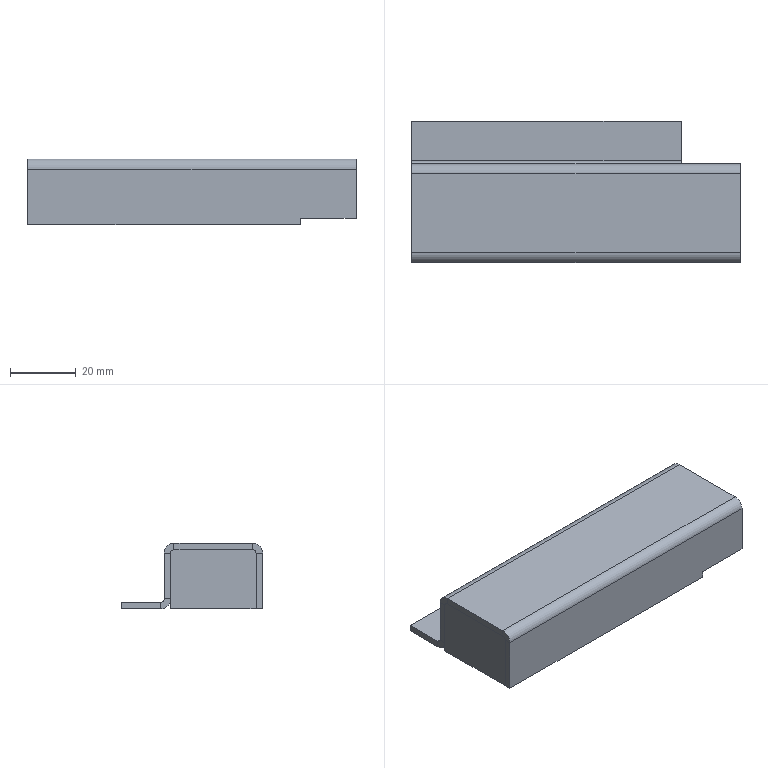Part | SolidWorks | features BaseBody 2 | 2 solids | 44 faces | box 100 x 43 x 20 mm | volume 15639 mm3 | plane 36 | cylinder 8 | commonest cylinder face diameters 2 x5 6 x3
STEP:
#1=CARTESIAN_POINT('',(33.,-13.,-20.));
#2=VERTEX_POINT('',#1);
#3=CARTESIAN_POINT('',(33.,-13.,-18.));
#4=VERTEX_POINT('',#3);
#5=CARTESIAN_POINT('',(33.,-13.,0.));
#6=DIRECTION('',(0.,0.,1.));
#7=VECTOR('',#6,1000.);
#8=LINE('',#5,#7);
#9=EDGE_CURVE('',#2,#4,#8,.T.);
#10=ORIENTED_EDGE('',*,*,#9,.T.);
#11=CARTESIAN_POINT('',(33.,-15.,-18.));
#12=VERTEX_POINT('',#11);
#13=CARTESIAN_POINT('',(33.,-15.,-18.));
#14=DIRECTION('',(0.,1.,0.));
#15=VECTOR('',#14,1000.);
#16=LINE('',#13,#15);
#17=EDGE_CURVE('',#12,#4,#16,.T.);
#18=ORIENTED_EDGE('',*,*,#17,.F.);
#19=CARTESIAN_POINT('',(33.,-15.,-20.));
#20=VERTEX_POINT('',#19);
#21=CARTESIAN_POINT('',(33.,-15.,-20.));
#22=DIRECTION('',(0.,0.,1.));
#23=VECTOR('',#22,1000.);
#24=LINE('',#21,#23);
#25=EDGE_CURVE('',#20,#12,#24,.T.);
#26=ORIENTED_EDGE('',*,*,#25,.F.);
#27=CARTESIAN_POINT('',(33.,-15.,-20.));
#28=DIRECTION('',(0.,1.,0.));
#29=VECTOR('',#28,1000.);
#30=LINE('',#27,#29);
#31=EDGE_CURVE('',#20,#2,#30,.T.);
#32=ORIENTED_EDGE('',*,*,#31,.T.);
#33=EDGE_LOOP('',(#10,#18,#26,#32));
#34=FACE_OUTER_BOUND('',#33,.T.);
#35=CARTESIAN_POINT('',(33.,-15.,-20.));
#36=DIRECTION('',(-1.,0.,0.));
#37=DIRECTION('',(0.,0.,1.));
#38=AXIS2_PLACEMENT_3D('',#35,#36,#37);
#39=PLANE('',#38);
#40=ADVANCED_FACE('',(#34),#39,.F.);
#41=CARTESIAN_POINT('',(50.,-13.,-18.));
#42=VERTEX_POINT('',#41);
#43=CARTESIAN_POINT('',(0.,-13.,-18.));
#44=DIRECTION('',(1.,0.,0.));
#45=VECTOR('',#44,1000.);
#46=LINE('',#43,#45);
#47=EDGE_CURVE('',#4,#42,#46,.T.);
#48=ORIENTED_EDGE('',*,*,#47,.T.);
#49=CARTESIAN_POINT('',(50.,-15.,-18.));
#50=VERTEX_POINT('',#49);
#51=CARTESIAN_POINT('',(50.,-15.,-18.));
#52=DIRECTION('',(0.,1.,0.));
#53=VECTOR('',#52,1000.);
#54=LINE('',#51,#53);
#55=EDGE_CURVE('',#50,#42,#54,.T.);
#56=ORIENTED_EDGE('',*,*,#55,.F.);
#57=CARTESIAN_POINT('',(50.,-15.,-18.));
#58=DIRECTION('',(1.,0.,0.));
#59=VECTOR('',#58,1000.);
#60=LINE('',#57,#59);
#61=EDGE_CURVE('',#12,#50,#60,.T.);
#62=ORIENTED_EDGE('',*,*,#61,.F.);
#63=ORIENTED_EDGE('',*,*,#17,.T.);
#64=EDGE_LOOP('',(#48,#56,#62,#63));
#65=FACE_OUTER_BOUND('',#64,.T.);
#66=CARTESIAN_POINT('',(50.,-15.,-18.));
#67=DIRECTION('',(0.,0.,1.));
#68=DIRECTION('',(0.,-1.,0.));
#69=AXIS2_PLACEMENT_3D('',#66,#67,#68);
#70=PLANE('',#69);
#71=ADVANCED_FACE('',(#65),#70,.F.);
#72=CARTESIAN_POINT('',(33.,13.,-18.));
#73=VERTEX_POINT('',#72);
#74=CARTESIAN_POINT('',(33.,15.,-18.));
#75=VERTEX_POINT('',#74);
#76=CARTESIAN_POINT('',(33.,15.,-18.));
#77=DIRECTION('',(0.,1.,0.));
#78=VECTOR('',#77,1000.);
#79=LINE('',#76,#78);
#80=EDGE_CURVE('',#73,#75,#79,.T.);
#81=ORIENTED_EDGE('',*,*,#80,.T.);
#82=CARTESIAN_POINT('',(50.,15.,-18.));
#83=VERTEX_POINT('',#82);
#84=CARTESIAN_POINT('',(50.,15.,-18.));
#85=DIRECTION('',(1.,0.,0.));
#86=VECTOR('',#85,1000.);
#87=LINE('',#84,#86);
#88=EDGE_CURVE('',#75,#83,#87,.T.);
#89=ORIENTED_EDGE('',*,*,#88,.T.);
#90=CARTESIAN_POINT('',(50.,13.,-18.));
#91=VERTEX_POINT('',#90);
#92=CARTESIAN_POINT('',(50.,-15.,-18.));
#93=DIRECTION('',(0.,1.,0.));
#94=VECTOR('',#93,1000.);
#95=LINE('',#92,#94);
#96=EDGE_CURVE('',#91,#83,#95,.T.);
#97=ORIENTED_EDGE('',*,*,#96,.F.);
#98=CARTESIAN_POINT('',(0.,13.,-18.));
#99=DIRECTION('',(1.,0.,0.));
#100=VECTOR('',#99,1000.);
#101=LINE('',#98,#100);
#102=EDGE_CURVE('',#73,#91,#101,.T.);
#103=ORIENTED_EDGE('',*,*,#102,.F.);
#104=EDGE_LOOP('',(#81,#89,#97,#103));
#105=FACE_OUTER_BOUND('',#104,.T.);
#106=CARTESIAN_POINT('',(50.,-15.,-18.));
#107=DIRECTION('',(0.,0.,1.));
#108=DIRECTION('',(0.,-1.,0.));
#109=AXIS2_PLACEMENT_3D('',#106,#107,#108);
#110=PLANE('',#109);
#111=ADVANCED_FACE('',(#105),#110,.F.);
#112=CARTESIAN_POINT('',(32.,28.,-18.));
#113=VERTEX_POINT('',#112);
#114=CARTESIAN_POINT('',(-50.,28.,-18.));
#115=VERTEX_POINT('',#114);
#116=CARTESIAN_POINT('',(0.,28.,-18.));
#117=DIRECTION('',(-1.,0.,0.));
#118=VECTOR('',#117,1000.);
#119=LINE('',#116,#118);
#120=EDGE_CURVE('',#113,#115,#119,.T.);
#121=ORIENTED_EDGE('',*,*,#120,.F.);
#122=CARTESIAN_POINT('',(32.,28.,-20.));
#123=VERTEX_POINT('',#122);
#124=CARTESIAN_POINT('',(32.,28.,-20.));
#125=DIRECTION('',(0.,0.,1.));
#126=VECTOR('',#125,1000.);
#127=LINE('',#124,#126);
#128=EDGE_CURVE('',#123,#113,#127,.T.);
#129=ORIENTED_EDGE('',*,*,#128,.F.);
#130=CARTESIAN_POINT('',(-50.,28.,-20.));
#131=VERTEX_POINT('',#130);
#132=CARTESIAN_POINT('',(-50.,28.,-20.));
#133=DIRECTION('',(-1.,0.,0.));
#134=VECTOR('',#133,1000.);
#135=LINE('',#132,#134);
#136=EDGE_CURVE('',#123,#131,#135,.T.);
#137=ORIENTED_EDGE('',*,*,#136,.T.);
#138=CARTESIAN_POINT('',(-50.,28.,-20.));
#139=DIRECTION('',(0.,0.,1.));
#140=VECTOR('',#139,1000.);
#141=LINE('',#138,#140);
#142=EDGE_CURVE('',#131,#115,#141,.T.);
#143=ORIENTED_EDGE('',*,*,#142,.T.);
#144=EDGE_LOOP('',(#121,#129,#137,#143));
#145=FACE_OUTER_BOUND('',#144,.T.);
#146=CARTESIAN_POINT('',(-50.,28.,-20.));
#147=DIRECTION('',(0.,1.,0.));
#148=DIRECTION('',(1.,0.,0.));
#149=AXIS2_PLACEMENT_3D('',#146,#147,#148);
#150=PLANE('',#149);
#151=ADVANCED_FACE('',(#145),#150,.T.);
#152=CARTESIAN_POINT('',(32.,16.,-18.));
#153=VERTEX_POINT('',#152);
#154=CARTESIAN_POINT('',(-50.,16.,-18.));
#155=VERTEX_POINT('',#154);
#156=CARTESIAN_POINT('',(32.,16.,-18.));
#157=DIRECTION('',(-1.,0.,0.));
#158=VECTOR('',#157,1000.);
#159=LINE('',#156,#158);
#160=EDGE_CURVE('',#153,#155,#159,.T.);
#161=ORIENTED_EDGE('',*,*,#160,.F.);
#162=CARTESIAN_POINT('',(32.,0.,-18.));
#163=DIRECTION('',(0.,1.,0.));
#164=VECTOR('',#163,1000.);
#165=LINE('',#162,#164);
#166=EDGE_CURVE('',#153,#113,#165,.T.);
#167=ORIENTED_EDGE('',*,*,#166,.T.);
#168=ORIENTED_EDGE('',*,*,#120,.T.);
#169=CARTESIAN_POINT('',(-50.,0.,-18.));
#170=DIRECTION('',(0.,-1.,0.));
#171=VECTOR('',#170,1000.);
#172=LINE('',#169,#171);
#173=EDGE_CURVE('',#115,#155,#172,.T.);
#174=ORIENTED_EDGE('',*,*,#173,.T.);
#175=EDGE_LOOP('',(#161,#167,#168,#174));
#176=FACE_OUTER_BOUND('',#175,.T.);
#177=CARTESIAN_POINT('',(0.,0.,-18.));
#178=DIRECTION('',(0.,0.,-1.));
#179=DIRECTION('',(0.,-1.,0.));
#180=AXIS2_PLACEMENT_3D('',#177,#178,#179);
#181=PLANE('',#180);
#182=ADVANCED_FACE('',(#176),#181,.F.);
#183=CARTESIAN_POINT('',(32.,16.,-20.));
#184=VERTEX_POINT('',#183);
#185=CARTESIAN_POINT('',(32.,15.,-20.));
#186=DIRECTION('',(0.,1.,0.));
#187=VECTOR('',#186,1000.);
#188=LINE('',#185,#187);
#189=EDGE_CURVE('',#184,#123,#188,.T.);
#190=ORIENTED_EDGE('',*,*,#189,.F.);
#191=CARTESIAN_POINT('',(-50.,16.,-20.));
#192=VERTEX_POINT('',#191);
#193=CARTESIAN_POINT('',(0.,16.,-20.));
#194=DIRECTION('',(-1.,0.,0.));
#195=VECTOR('',#194,1000.);
#196=LINE('',#193,#195);
#197=EDGE_CURVE('',#184,#192,#196,.T.);
#198=ORIENTED_EDGE('',*,*,#197,.T.);
#199=CARTESIAN_POINT('',(-50.,15.,-20.));
#200=DIRECTION('',(0.,-1.,0.));
#201=VECTOR('',#200,1000.);
#202=LINE('',#199,#201);
#203=EDGE_CURVE('',#131,#192,#202,.T.);
#204=ORIENTED_EDGE('',*,*,#203,.F.);
#205=ORIENTED_EDGE('',*,*,#136,.F.);
#206=EDGE_LOOP('',(#190,#198,#204,#205));
#207=FACE_OUTER_BOUND('',#206,.T.);
#208=CARTESIAN_POINT('',(0.,0.,-20.));
#209=DIRECTION('',(0.,0.,-1.));
#210=DIRECTION('',(0.,-1.,0.));
#211=AXIS2_PLACEMENT_3D('',#208,#209,#210);
#212=PLANE('',#211);
#213=ADVANCED_FACE('',(#207),#212,.T.);
#214=ORIENTED_EDGE('',*,*,#166,.F.);
#215=CARTESIAN_POINT('',(32.,16.,-20.));
#216=DIRECTION('',(0.,0.,-1.));
#217=VECTOR('',#216,1000.);
#218=LINE('',#215,#217);
#219=EDGE_CURVE('',#153,#184,#218,.T.);
#220=ORIENTED_EDGE('',*,*,#219,.T.);
#221=ORIENTED_EDGE('',*,*,#189,.T.);
#222=ORIENTED_EDGE('',*,*,#128,.T.);
#223=EDGE_LOOP('',(#214,#220,#221,#222));
#224=FACE_OUTER_BOUND('',#223,.T.);
#225=CARTESIAN_POINT('',(32.,15.,-20.));
#226=DIRECTION('',(1.,0.,0.));
#227=DIRECTION('',(0.,1.,0.));
#228=AXIS2_PLACEMENT_3D('',#225,#226,#227);
#229=PLANE('',#228);
#230=ADVANCED_FACE('',(#224),#229,.T.);
#231=ORIENTED_EDGE('',*,*,#203,.T.);
#232=CARTESIAN_POINT('',(-50.,16.,-18.));
#233=DIRECTION('',(0.,0.,-1.));
#234=VECTOR('',#233,1000.);
#235=LINE('',#232,#234);
#236=EDGE_CURVE('',#155,#192,#235,.T.);
#237=ORIENTED_EDGE('',*,*,#236,.F.);
#238=ORIENTED_EDGE('',*,*,#173,.F.);
#239=ORIENTED_EDGE('',*,*,#142,.F.);
#240=EDGE_LOOP('',(#231,#237,#238,#239));
#241=FACE_OUTER_BOUND('',#240,.T.);
#242=CARTESIAN_POINT('',(-50.,15.,-20.));
#243=DIRECTION('',(-1.,0.,0.));
#244=DIRECTION('',(0.,0.,1.));
#245=AXIS2_PLACEMENT_3D('',#242,#243,#244);
#246=PLANE('',#245);
#247=ADVANCED_FACE('',(#241),#246,.T.);
#248=CARTESIAN_POINT('',(-50.,15.,-17.));
#249=VERTEX_POINT('',#248);
#250=CARTESIAN_POINT('',(32.,15.,-17.));
#251=VERTEX_POINT('',#250);
#252=CARTESIAN_POINT('',(-50.,15.,-17.));
#253=DIRECTION('',(1.,0.,0.));
#254=VECTOR('',#253,1000.);
#255=LINE('',#252,#254);
#256=EDGE_CURVE('',#249,#251,#255,.T.);
#257=ORIENTED_EDGE('',*,*,#256,.T.);
#258=CARTESIAN_POINT('',(32.,16.,-17.));
#259=DIRECTION('',(1.,0.,0.));
#260=DIRECTION('',(0.,0.,1.));
#261=AXIS2_PLACEMENT_3D('',#258,#259,#260);
#262=CIRCLE('',#261,1.);
#263=EDGE_CURVE('',#251,#153,#262,.T.);
#264=ORIENTED_EDGE('',*,*,#263,.T.);
#265=ORIENTED_EDGE('',*,*,#160,.T.);
#266=CARTESIAN_POINT('',(-50.,16.,-17.));
#267=DIRECTION('',(-1.,0.,0.));
#268=DIRECTION('',(0.,0.,1.));
#269=AXIS2_PLACEMENT_3D('',#266,#267,#268);
#270=CIRCLE('',#269,1.);
#271=EDGE_CURVE('',#155,#249,#270,.T.);
#272=ORIENTED_EDGE('',*,*,#271,.T.);
#273=EDGE_LOOP('',(#257,#264,#265,#272));
#274=FACE_OUTER_BOUND('',#273,.T.);
#275=CARTESIAN_POINT('',(-50.,16.,-17.));
#276=DIRECTION('',(-1.,0.,0.));
#277=DIRECTION('',(0.,0.,-1.));
#278=AXIS2_PLACEMENT_3D('',#275,#276,#277);
#279=CYLINDRICAL_SURFACE('',#278,1.);
#280=ADVANCED_FACE('',(#274),#279,.F.);
#281=CARTESIAN_POINT('',(-50.,13.,-17.));
#282=VERTEX_POINT('',#281);
#283=CARTESIAN_POINT('',(32.,13.,-17.));
#284=VERTEX_POINT('',#283);
#285=CARTESIAN_POINT('',(-50.,13.,-17.));
#286=DIRECTION('',(1.,0.,0.));
#287=VECTOR('',#286,1000.);
#288=LINE('',#285,#287);
#289=EDGE_CURVE('',#282,#284,#288,.T.);
#290=ORIENTED_EDGE('',*,*,#289,.F.);
#291=CARTESIAN_POINT('',(-50.,16.,-17.));
#292=DIRECTION('',(-1.,0.,0.));
#293=DIRECTION('',(0.,0.,1.));
#294=AXIS2_PLACEMENT_3D('',#291,#292,#293);
#295=CIRCLE('',#294,3.);
#296=EDGE_CURVE('',#192,#282,#295,.T.);
#297=ORIENTED_EDGE('',*,*,#296,.F.);
#298=ORIENTED_EDGE('',*,*,#197,.F.);
#299=CARTESIAN_POINT('',(32.,16.,-17.));
#300=DIRECTION('',(1.,0.,0.));
#301=DIRECTION('',(0.,0.,1.));
#302=AXIS2_PLACEMENT_3D('',#299,#300,#301);
#303=CIRCLE('',#302,3.);
#304=EDGE_CURVE('',#284,#184,#303,.T.);
#305=ORIENTED_EDGE('',*,*,#304,.F.);
#306=EDGE_LOOP('',(#290,#297,#298,#305));
#307=FACE_OUTER_BOUND('',#306,.T.);
#308=CARTESIAN_POINT('',(-50.,16.,-17.));
#309=DIRECTION('',(-1.,0.,0.));
#310=DIRECTION('',(0.,0.,-1.));
#311=AXIS2_PLACEMENT_3D('',#308,#309,#310);
#312=CYLINDRICAL_SURFACE('',#311,3.);
#313=ADVANCED_FACE('',(#307),#312,.T.);
#314=ORIENTED_EDGE('',*,*,#271,.F.);
#315=ORIENTED_EDGE('',*,*,#236,.T.);
#316=ORIENTED_EDGE('',*,*,#296,.T.);
#317=CARTESIAN_POINT('',(-50.,15.,-17.));
#318=DIRECTION('',(0.,-1.,0.));
#319=VECTOR('',#318,1000.);
#320=LINE('',#317,#319);
#321=EDGE_CURVE('',#249,#282,#320,.T.);
#322=ORIENTED_EDGE('',*,*,#321,.F.);
#323=EDGE_LOOP('',(#314,#315,#316,#322));
#324=FACE_OUTER_BOUND('',#323,.T.);
#325=CARTESIAN_POINT('',(-50.,16.,-17.));
#326=DIRECTION('',(1.,0.,0.));
#327=DIRECTION('',(0.,1.,0.));
#328=AXIS2_PLACEMENT_3D('',#325,#326,#327);
#329=PLANE('',#328);
#330=ADVANCED_FACE('',(#324),#329,.F.);
#331=ORIENTED_EDGE('',*,*,#219,.F.);
#332=ORIENTED_EDGE('',*,*,#263,.F.);
#333=CARTESIAN_POINT('',(32.,15.,-17.));
#334=DIRECTION('',(0.,-1.,0.));
#335=VECTOR('',#334,1000.);
#336=LINE('',#333,#335);
#337=EDGE_CURVE('',#251,#284,#336,.T.);
#338=ORIENTED_EDGE('',*,*,#337,.T.);
#339=ORIENTED_EDGE('',*,*,#304,.T.);
#340=EDGE_LOOP('',(#331,#332,#338,#339));
#341=FACE_OUTER_BOUND('',#340,.T.);
#342=CARTESIAN_POINT('',(32.,16.,-17.));
#343=DIRECTION('',(1.,0.,0.));
#344=DIRECTION('',(0.,1.,0.));
#345=AXIS2_PLACEMENT_3D('',#342,#343,#344);
#346=PLANE('',#345);
#347=ADVANCED_FACE('',(#341),#346,.T.);
#348=ORIENTED_EDGE('',*,*,#80,.F.);
#349=CARTESIAN_POINT('',(33.,13.,-16.));
#350=VERTEX_POINT('',#349);
#351=CARTESIAN_POINT('',(33.,13.,0.));
#352=DIRECTION('',(0.,0.,1.));
#353=VECTOR('',#352,1000.);
#354=LINE('',#351,#353);
#355=EDGE_CURVE('',#73,#350,#354,.T.);
#356=ORIENTED_EDGE('',*,*,#355,.T.);
#357=CARTESIAN_POINT('',(33.,15.,-16.));
#358=VERTEX_POINT('',#357);
#359=CARTESIAN_POINT('',(33.,15.,-16.));
#360=DIRECTION('',(0.,-1.,0.));
#361=VECTOR('',#360,1000.);
#362=LINE('',#359,#361);
#363=EDGE_CURVE('',#358,#350,#362,.T.);
#364=ORIENTED_EDGE('',*,*,#363,.F.);
#365=CARTESIAN_POINT('',(33.,15.,-16.));
#366=DIRECTION('',(0.,0.,-1.));
#367=VECTOR('',#366,1000.);
#368=LINE('',#365,#367);
#369=EDGE_CURVE('',#358,#75,#368,.T.);
#370=ORIENTED_EDGE('',*,*,#369,.T.);
#371=EDGE_LOOP('',(#348,#356,#364,#370));
#372=FACE_OUTER_BOUND('',#371,.T.);
#373=CARTESIAN_POINT('',(33.,15.,-16.));
#374=DIRECTION('',(-1.,0.,0.));
#375=DIRECTION('',(0.,0.,1.));
#376=AXIS2_PLACEMENT_3D('',#373,#374,#375);
#377=PLANE('',#376);
#378=ADVANCED_FACE('',(#372),#377,.T.);
#379=ORIENTED_EDGE('',*,*,#363,.T.);
#380=CARTESIAN_POINT('',(32.,13.,-16.));
#381=VERTEX_POINT('',#380);
#382=CARTESIAN_POINT('',(0.,13.,-16.));
#383=DIRECTION('',(-1.,0.,0.));
#384=VECTOR('',#383,1000.);
#385=LINE('',#382,#384);
#386=EDGE_CURVE('',#350,#381,#385,.T.);
#387=ORIENTED_EDGE('',*,*,#386,.T.);
#388=CARTESIAN_POINT('',(32.,15.,-16.));
#389=VERTEX_POINT('',#388);
#390=CARTESIAN_POINT('',(32.,15.,-16.));
#391=DIRECTION('',(0.,-1.,0.));
#392=VECTOR('',#391,1000.);
#393=LINE('',#390,#392);
#394=EDGE_CURVE('',#389,#381,#393,.T.);
#395=ORIENTED_EDGE('',*,*,#394,.F.);
#396=CARTESIAN_POINT('',(32.,15.,-16.));
#397=DIRECTION('',(1.,0.,0.));
#398=VECTOR('',#397,1000.);
#399=LINE('',#396,#398);
#400=EDGE_CURVE('',#389,#358,#399,.T.);
#401=ORIENTED_EDGE('',*,*,#400,.T.);
#402=EDGE_LOOP('',(#379,#387,#395,#401));
#403=FACE_OUTER_BOUND('',#402,.T.);
#404=CARTESIAN_POINT('',(32.,15.,-16.));
#405=DIRECTION('',(0.,0.,-1.));
#406=DIRECTION('',(-1.,0.,0.));
#407=AXIS2_PLACEMENT_3D('',#404,#405,#406);
#408=PLANE('',#407);
#409=ADVANCED_FACE('',(#403),#408,.T.);
#410=ORIENTED_EDGE('',*,*,#394,.T.);
#411=CARTESIAN_POINT('',(32.,13.,0.));
#412=DIRECTION('',(0.,0.,-1.));
#413=VECTOR('',#412,1000.);
#414=LINE('',#411,#413);
#415=EDGE_CURVE('',#381,#284,#414,.T.);
#416=ORIENTED_EDGE('',*,*,#415,.T.);
#417=ORIENTED_EDGE('',*,*,#337,.F.);
#418=CARTESIAN_POINT('',(32.,15.,-17.));
#419=DIRECTION('',(0.,0.,1.));
#420=VECTOR('',#419,1000.);
#421=LINE('',#418,#420);
#422=EDGE_CURVE('',#251,#389,#421,.T.);
#423=ORIENTED_EDGE('',*,*,#422,.T.);
#424=EDGE_LOOP('',(#410,#416,#417,#423));
#425=FACE_OUTER_BOUND('',#424,.T.);
#426=CARTESIAN_POINT('',(32.,15.,-17.));
#427=DIRECTION('',(1.,0.,0.));
#428=DIRECTION('',(0.,1.,0.));
#429=AXIS2_PLACEMENT_3D('',#426,#427,#428);
#430=PLANE('',#429);
#431=ADVANCED_FACE('',(#425),#430,.T.);
#432=ORIENTED_EDGE('',*,*,#31,.F.);
#433=CARTESIAN_POINT('',(-50.,-15.,-20.));
#434=VERTEX_POINT('',#433);
#435=CARTESIAN_POINT('',(50.,-15.,-20.));
#436=DIRECTION('',(-1.,0.,0.));
#437=VECTOR('',#436,1000.);
#438=LINE('',#435,#437);
#439=EDGE_CURVE('',#20,#434,#438,.T.);
#440=ORIENTED_EDGE('',*,*,#439,.T.);
#441=CARTESIAN_POINT('',(-50.,-13.,-20.));
#442=VERTEX_POINT('',#441);
#443=CARTESIAN_POINT('',(-50.,-15.,-20.));
#444=DIRECTION('',(0.,1.,0.));
#445=VECTOR('',#444,1000.);
#446=LINE('',#443,#445);
#447=EDGE_CURVE('',#434,#442,#446,.T.);
#448=ORIENTED_EDGE('',*,*,#447,.T.);
#449=CARTESIAN_POINT('',(0.,-13.,-20.));
#450=DIRECTION('',(-1.,0.,0.));
#451=VECTOR('',#450,1000.);
#452=LINE('',#449,#451);
#453=EDGE_CURVE('',#2,#442,#452,.T.);
#454=ORIENTED_EDGE('',*,*,#453,.F.);
#455=EDGE_LOOP('',(#432,#440,#448,#454));
#456=FACE_OUTER_BOUND('',#455,.T.);
#457=CARTESIAN_POINT('',(50.,-15.,-20.));
#458=DIRECTION('',(0.,0.,-1.));
#459=DIRECTION('',(0.,-1.,0.));
#460=AXIS2_PLACEMENT_3D('',#457,#458,#459);
#461=PLANE('',#460);
#462=ADVANCED_FACE('',(#456),#461,.T.);
#463=ORIENTED_EDGE('',*,*,#47,.F.);
#464=ORIENTED_EDGE('',*,*,#9,.F.);
#465=ORIENTED_EDGE('',*,*,#453,.T.);
#466=CARTESIAN_POINT('',(-50.,-13.,-3.));
#467=VERTEX_POINT('',#466);
#468=CARTESIAN_POINT('',(-50.,-13.,0.));
#469=DIRECTION('',(0.,0.,1.));
#470=VECTOR('',#469,1000.);
#471=LINE('',#468,#470);
#472=EDGE_CURVE('',#442,#467,#471,.T.);
#473=ORIENTED_EDGE('',*,*,#472,.T.);
#474=CARTESIAN_POINT('',(50.,-13.,-3.));
#475=VERTEX_POINT('',#474);
#476=CARTESIAN_POINT('',(50.,-13.,-3.));
#477=DIRECTION('',(-1.,0.,0.));
#478=VECTOR('',#477,1000.);
#479=LINE('',#476,#478);
#480=EDGE_CURVE('',#475,#467,#479,.T.);
#481=ORIENTED_EDGE('',*,*,#480,.F.);
#482=CARTESIAN_POINT('',(50.,-13.,0.));
#483=DIRECTION('',(0.,0.,-1.));
#484=VECTOR('',#483,1000.);
#485=LINE('',#482,#484);
#486=EDGE_CURVE('',#475,#42,#485,.T.);
#487=ORIENTED_EDGE('',*,*,#486,.T.);
#488=EDGE_LOOP('',(#463,#464,#465,#473,#481,#487));
#489=FACE_OUTER_BOUND('',#488,.T.);
#490=CARTESIAN_POINT('',(0.,-13.,0.));
#491=DIRECTION('',(0.,1.,0.));
#492=DIRECTION('',(0.,0.,-1.));
#493=AXIS2_PLACEMENT_3D('',#490,#491,#492);
#494=PLANE('',#493);
#495=ADVANCED_FACE('',(#489),#494,.T.);
#496=ORIENTED_EDGE('',*,*,#25,.T.);
#497=ORIENTED_EDGE('',*,*,#61,.T.);
#498=CARTESIAN_POINT('',(50.,-15.,-3.));
#499=VERTEX_POINT('',#498);
#500=CARTESIAN_POINT('',(50.,-15.,-2.));
#501=DIRECTION('',(0.,0.,-1.));
#502=VECTOR('',#501,1000.);
#503=LINE('',#500,#502);
#504=EDGE_CURVE('',#499,#50,#503,.T.);
#505=ORIENTED_EDGE('',*,*,#504,.F.);
#506=CARTESIAN_POINT('',(-50.,-15.,-3.));
#507=VERTEX_POINT('',#506);
#508=CARTESIAN_POINT('',(50.,-15.,-3.));
#509=DIRECTION('',(1.,0.,0.));
#510=VECTOR('',#509,1000.);
#511=LINE('',#508,#510);
#512=EDGE_CURVE('',#507,#499,#511,.T.);
#513=ORIENTED_EDGE('',*,*,#512,.F.);
#514=CARTESIAN_POINT('',(-50.,-15.,-20.));
#515=DIRECTION('',(0.,0.,1.));
#516=VECTOR('',#515,1000.);
#517=LINE('',#514,#516);
#518=EDGE_CURVE('',#434,#507,#517,.T.);
#519=ORIENTED_EDGE('',*,*,#518,.F.);
#520=ORIENTED_EDGE('',*,*,#439,.F.);
#521=EDGE_LOOP('',(#496,#497,#505,#513,#519,#520));
#522=FACE_OUTER_BOUND('',#521,.T.);
#523=CARTESIAN_POINT('',(0.,-15.,0.));
#524=DIRECTION('',(0.,1.,0.));
#525=DIRECTION('',(0.,0.,-1.));
#526=AXIS2_PLACEMENT_3D('',#523,#524,#525);
#527=PLANE('',#526);
#528=ADVANCED_FACE('',(#522),#527,.F.);
#529=ORIENTED_EDGE('',*,*,#518,.T.);
#530=CARTESIAN_POINT('',(-50.,-13.,-3.));
#531=DIRECTION('',(0.,-1.,0.));
#532=VECTOR('',#531,1000.);
#533=LINE('',#530,#532);
#534=EDGE_CURVE('',#467,#507,#533,.T.);
#535=ORIENTED_EDGE('',*,*,#534,.F.);
#536=ORIENTED_EDGE('',*,*,#472,.F.);
#537=ORIENTED_EDGE('',*,*,#447,.F.);
#538=EDGE_LOOP('',(#529,#535,#536,#537));
#539=FACE_OUTER_BOUND('',#538,.T.);
#540=CARTESIAN_POINT('',(-50.,-15.,-20.));
#541=DIRECTION('',(-1.,0.,0.));
#542=DIRECTION('',(0.,0.,1.));
#543=AXIS2_PLACEMENT_3D('',#540,#541,#542);
#544=PLANE('',#543);
#545=ADVANCED_FACE('',(#539),#544,.T.);
#546=ORIENTED_EDGE('',*,*,#55,.T.);
#547=ORIENTED_EDGE('',*,*,#486,.F.);
#548=CARTESIAN_POINT('',(50.,-15.,-3.));
#549=DIRECTION('',(0.,-1.,0.));
#550=VECTOR('',#549,1000.);
#551=LINE('',#548,#550);
#552=EDGE_CURVE('',#475,#499,#551,.T.);
#553=ORIENTED_EDGE('',*,*,#552,.T.);
#554=ORIENTED_EDGE('',*,*,#504,.T.);
#555=EDGE_LOOP('',(#546,#547,#553,#554));
#556=FACE_OUTER_BOUND('',#555,.T.);
#557=CARTESIAN_POINT('',(50.,-15.,-2.));
#558=DIRECTION('',(1.,0.,0.));
#559=DIRECTION('',(0.,1.,0.));
#560=AXIS2_PLACEMENT_3D('',#557,#558,#559);
#561=PLANE('',#560);
#562=ADVANCED_FACE('',(#556),#561,.T.);
#563=CARTESIAN_POINT('',(-50.,-12.,-2.));
#564=VERTEX_POINT('',#563);
#565=CARTESIAN_POINT('',(50.,-12.,-2.));
#566=VERTEX_POINT('',#565);
#567=CARTESIAN_POINT('',(-50.,-12.,-2.));
#568=DIRECTION('',(1.,0.,0.));
#569=VECTOR('',#568,1000.);
#570=LINE('',#567,#569);
#571=EDGE_CURVE('',#564,#566,#570,.T.);
#572=ORIENTED_EDGE('',*,*,#571,.T.);
#573=CARTESIAN_POINT('',(50.,-12.,-3.));
#574=DIRECTION('',(1.,0.,0.));
#575=DIRECTION('',(0.,0.,1.));
#576=AXIS2_PLACEMENT_3D('',#573,#574,#575);
#577=CIRCLE('',#576,1.);
#578=EDGE_CURVE('',#566,#475,#577,.T.);
#579=ORIENTED_EDGE('',*,*,#578,.T.);
#580=ORIENTED_EDGE('',*,*,#480,.T.);
#581=CARTESIAN_POINT('',(-50.,-12.,-3.));
#582=DIRECTION('',(-1.,0.,0.));
#583=DIRECTION('',(0.,0.,1.));
#584=AXIS2_PLACEMENT_3D('',#581,#582,#583);
#585=CIRCLE('',#584,1.);
#586=EDGE_CURVE('',#467,#564,#585,.T.);
#587=ORIENTED_EDGE('',*,*,#586,.T.);
#588=EDGE_LOOP('',(#572,#579,#580,#587));
#589=FACE_OUTER_BOUND('',#588,.T.);
#590=CARTESIAN_POINT('',(-50.,-12.,-3.));
#591=DIRECTION('',(-1.,0.,0.));
#592=DIRECTION('',(0.,-1.,0.));
#593=AXIS2_PLACEMENT_3D('',#590,#591,#592);
#594=CYLINDRICAL_SURFACE('',#593,1.);
#595=ADVANCED_FACE('',(#589),#594,.F.);
#596=CARTESIAN_POINT('',(-50.,-12.,0.));
#597=VERTEX_POINT('',#596);
#598=CARTESIAN_POINT('',(50.,-12.,0.));
#599=VERTEX_POINT('',#598);
#600=CARTESIAN_POINT('',(-50.,-12.,0.));
#601=DIRECTION('',(1.,0.,0.));
#602=VECTOR('',#601,1000.);
#603=LINE('',#600,#602);
#604=EDGE_CURVE('',#597,#599,#603,.T.);
#605=ORIENTED_EDGE('',*,*,#604,.F.);
#606=CARTESIAN_POINT('',(-50.,-12.,-3.));
#607=DIRECTION('',(-1.,0.,0.));
#608=DIRECTION('',(0.,0.,1.));
#609=AXIS2_PLACEMENT_3D('',#606,#607,#608);
#610=CIRCLE('',#609,3.);
#611=EDGE_CURVE('',#507,#597,#610,.T.);
#612=ORIENTED_EDGE('',*,*,#611,.F.);
#613=ORIENTED_EDGE('',*,*,#512,.T.);
#614=CARTESIAN_POINT('',(50.,-12.,-3.));
#615=DIRECTION('',(1.,0.,0.));
#616=DIRECTION('',(0.,0.,1.));
#617=AXIS2_PLACEMENT_3D('',#614,#615,#616);
#618=CIRCLE('',#617,3.);
#619=EDGE_CURVE('',#599,#499,#618,.T.);
#620=ORIENTED_EDGE('',*,*,#619,.F.);
#621=EDGE_LOOP('',(#605,#612,#613,#620));
#622=FACE_OUTER_BOUND('',#621,.T.);
#623=CARTESIAN_POINT('',(-50.,-12.,-3.));
#624=DIRECTION('',(-1.,0.,0.));
#625=DIRECTION('',(0.,-1.,0.));
#626=AXIS2_PLACEMENT_3D('',#623,#624,#625);
#627=CYLINDRICAL_SURFACE('',#626,3.);
#628=ADVANCED_FACE('',(#622),#627,.T.);
#629=ORIENTED_EDGE('',*,*,#586,.F.);
#630=ORIENTED_EDGE('',*,*,#534,.T.);
#631=ORIENTED_EDGE('',*,*,#611,.T.);
#632=CARTESIAN_POINT('',(-50.,-12.,-2.));
#633=DIRECTION('',(0.,0.,1.));
#634=VECTOR('',#633,1000.);
#635=LINE('',#632,#634);
#636=EDGE_CURVE('',#564,#597,#635,.T.);
#637=ORIENTED_EDGE('',*,*,#636,.F.);
#638=EDGE_LOOP('',(#629,#630,#631,#637));
#639=FACE_OUTER_BOUND('',#638,.T.);
#640=CARTESIAN_POINT('',(-50.,-12.,-3.));
#641=DIRECTION('',(1.,0.,0.));
#642=DIRECTION('',(0.,1.,0.));
#643=AXIS2_PLACEMENT_3D('',#640,#641,#642);
#644=PLANE('',#643);
#645=ADVANCED_FACE('',(#639),#644,.F.);
#646=ORIENTED_EDGE('',*,*,#552,.F.);
#647=ORIENTED_EDGE('',*,*,#578,.F.);
#648=CARTESIAN_POINT('',(50.,-12.,-2.));
#649=DIRECTION('',(0.,0.,1.));
#650=VECTOR('',#649,1000.);
#651=LINE('',#648,#650);
#652=EDGE_CURVE('',#566,#599,#651,.T.);
#653=ORIENTED_EDGE('',*,*,#652,.T.);
#654=ORIENTED_EDGE('',*,*,#619,.T.);
#655=EDGE_LOOP('',(#646,#647,#653,#654));
#656=FACE_OUTER_BOUND('',#655,.T.);
#657=CARTESIAN_POINT('',(50.,-12.,-3.));
#658=DIRECTION('',(1.,0.,0.));
#659=DIRECTION('',(0.,1.,0.));
#660=AXIS2_PLACEMENT_3D('',#657,#658,#659);
#661=PLANE('',#660);
#662=ADVANCED_FACE('',(#656),#661,.T.);
#663=ORIENTED_EDGE('',*,*,#96,.T.);
#664=CARTESIAN_POINT('',(50.,15.,-3.));
#665=VERTEX_POINT('',#664);
#666=CARTESIAN_POINT('',(50.,15.,-2.));
#667=DIRECTION('',(0.,0.,1.));
#668=VECTOR('',#667,1000.);
#669=LINE('',#666,#668);
#670=EDGE_CURVE('',#83,#665,#669,.T.);
#671=ORIENTED_EDGE('',*,*,#670,.T.);
#672=CARTESIAN_POINT('',(50.,13.,-3.));
#673=VERTEX_POINT('',#672);
#674=CARTESIAN_POINT('',(50.,13.,-3.));
#675=DIRECTION('',(0.,1.,0.));
#676=VECTOR('',#675,1000.);
#677=LINE('',#674,#676);
#678=EDGE_CURVE('',#673,#665,#677,.T.);
#679=ORIENTED_EDGE('',*,*,#678,.F.);
#680=CARTESIAN_POINT('',(50.,13.,0.));
#681=DIRECTION('',(0.,0.,1.));
#682=VECTOR('',#681,1000.);
#683=LINE('',#680,#682);
#684=EDGE_CURVE('',#91,#673,#683,.T.);
#685=ORIENTED_EDGE('',*,*,#684,.F.);
#686=EDGE_LOOP('',(#663,#671,#679,#685));
#687=FACE_OUTER_BOUND('',#686,.T.);
#688=CARTESIAN_POINT('',(50.,15.,-2.));
#689=DIRECTION('',(1.,0.,0.));
#690=DIRECTION('',(0.,1.,0.));
#691=AXIS2_PLACEMENT_3D('',#688,#689,#690);
#692=PLANE('',#691);
#693=ADVANCED_FACE('',(#687),#692,.T.);
#694=CARTESIAN_POINT('',(50.,12.,-2.));
#695=VERTEX_POINT('',#694);
#696=CARTESIAN_POINT('',(-50.,12.,-2.));
#697=VERTEX_POINT('',#696);
#698=CARTESIAN_POINT('',(50.,12.,-2.));
#699=DIRECTION('',(-1.,0.,0.));
#700=VECTOR('',#699,1000.);
#701=LINE('',#698,#700);
#702=EDGE_CURVE('',#695,#697,#701,.T.);
#703=ORIENTED_EDGE('',*,*,#702,.T.);
#704=CARTESIAN_POINT('',(-50.,13.,-3.));
#705=VERTEX_POINT('',#704);
#706=CARTESIAN_POINT('',(-50.,12.,-3.));
#707=DIRECTION('',(-1.,0.,0.));
#708=DIRECTION('',(0.,0.,-1.));
#709=AXIS2_PLACEMENT_3D('',#706,#707,#708);
#710=CIRCLE('',#709,1.);
#711=EDGE_CURVE('',#697,#705,#710,.T.);
#712=ORIENTED_EDGE('',*,*,#711,.T.);
#713=CARTESIAN_POINT('',(-50.,13.,-3.));
#714=DIRECTION('',(1.,0.,0.));
#715=VECTOR('',#714,1000.);
#716=LINE('',#713,#715);
#717=EDGE_CURVE('',#705,#673,#716,.T.);
#718=ORIENTED_EDGE('',*,*,#717,.T.);
#719=CARTESIAN_POINT('',(50.,12.,-3.));
#720=DIRECTION('',(1.,0.,0.));
#721=DIRECTION('',(0.,0.,-1.));
#722=AXIS2_PLACEMENT_3D('',#719,#720,#721);
#723=CIRCLE('',#722,1.);
#724=EDGE_CURVE('',#673,#695,#723,.T.);
#725=ORIENTED_EDGE('',*,*,#724,.T.);
#726=EDGE_LOOP('',(#703,#712,#718,#725));
#727=FACE_OUTER_BOUND('',#726,.T.);
#728=CARTESIAN_POINT('',(50.,12.,-3.));
#729=DIRECTION('',(1.,0.,0.));
#730=DIRECTION('',(0.,1.,0.));
#731=AXIS2_PLACEMENT_3D('',#728,#729,#730);
#732=CYLINDRICAL_SURFACE('',#731,1.);
#733=ADVANCED_FACE('',(#727),#732,.F.);
#734=CARTESIAN_POINT('',(50.,12.,0.));
#735=VERTEX_POINT('',#734);
#736=CARTESIAN_POINT('',(-50.,12.,0.));
#737=VERTEX_POINT('',#736);
#738=CARTESIAN_POINT('',(50.,12.,0.));
#739=DIRECTION('',(-1.,0.,0.));
#740=VECTOR('',#739,1000.);
#741=LINE('',#738,#740);
#742=EDGE_CURVE('',#735,#737,#741,.T.);
#743=ORIENTED_EDGE('',*,*,#742,.F.);
#744=CARTESIAN_POINT('',(50.,12.,-3.));
#745=DIRECTION('',(1.,0.,0.));
#746=DIRECTION('',(0.,0.,-1.));
#747=AXIS2_PLACEMENT_3D('',#744,#745,#746);
#748=CIRCLE('',#747,3.);
#749=EDGE_CURVE('',#665,#735,#748,.T.);
#750=ORIENTED_EDGE('',*,*,#749,.F.);
#751=CARTESIAN_POINT('',(-50.,15.,-3.));
#752=VERTEX_POINT('',#751);
#753=CARTESIAN_POINT('',(0.,15.,-3.));
#754=DIRECTION('',(1.,0.,0.));
#755=VECTOR('',#754,1000.);
#756=LINE('',#753,#755);
#757=EDGE_CURVE('',#752,#665,#756,.T.);
#758=ORIENTED_EDGE('',*,*,#757,.F.);
#759=CARTESIAN_POINT('',(-50.,12.,-3.));
#760=DIRECTION('',(-1.,0.,0.));
#761=DIRECTION('',(0.,0.,-1.));
#762=AXIS2_PLACEMENT_3D('',#759,#760,#761);
#763=CIRCLE('',#762,3.);
#764=EDGE_CURVE('',#737,#752,#763,.T.);
#765=ORIENTED_EDGE('',*,*,#764,.F.);
#766=EDGE_LOOP('',(#743,#750,#758,#765));
#767=FACE_OUTER_BOUND('',#766,.T.);
#768=CARTESIAN_POINT('',(50.,12.,-3.));
#769=DIRECTION('',(1.,0.,0.));
#770=DIRECTION('',(0.,1.,0.));
#771=AXIS2_PLACEMENT_3D('',#768,#769,#770);
#772=CYLINDRICAL_SURFACE('',#771,3.);
#773=ADVANCED_FACE('',(#767),#772,.T.);
#774=ORIENTED_EDGE('',*,*,#724,.F.);
#775=ORIENTED_EDGE('',*,*,#678,.T.);
#776=ORIENTED_EDGE('',*,*,#749,.T.);
#777=CARTESIAN_POINT('',(50.,12.,-2.));
#778=DIRECTION('',(0.,0.,1.));
#779=VECTOR('',#778,1000.);
#780=LINE('',#777,#779);
#781=EDGE_CURVE('',#695,#735,#780,.T.);
#782=ORIENTED_EDGE('',*,*,#781,.F.);
#783=EDGE_LOOP('',(#774,#775,#776,#782));
#784=FACE_OUTER_BOUND('',#783,.T.);
#785=CARTESIAN_POINT('',(50.,12.,-3.));
#786=DIRECTION('',(-1.,0.,0.));
#787=DIRECTION('',(0.,0.,1.));
#788=AXIS2_PLACEMENT_3D('',#785,#786,#787);
#789=PLANE('',#788);
#790=ADVANCED_FACE('',(#784),#789,.F.);
#791=CARTESIAN_POINT('',(-50.,15.,-3.));
#792=DIRECTION('',(0.,1.,0.));
#793=VECTOR('',#792,1000.);
#794=LINE('',#791,#793);
#795=EDGE_CURVE('',#705,#752,#794,.T.);
#796=ORIENTED_EDGE('',*,*,#795,.F.);
#797=ORIENTED_EDGE('',*,*,#711,.F.);
#798=CARTESIAN_POINT('',(-50.,12.,-2.));
#799=DIRECTION('',(0.,0.,1.));
#800=VECTOR('',#799,1000.);
#801=LINE('',#798,#800);
#802=EDGE_CURVE('',#697,#737,#801,.T.);
#803=ORIENTED_EDGE('',*,*,#802,.T.);
#804=ORIENTED_EDGE('',*,*,#764,.T.);
#805=EDGE_LOOP('',(#796,#797,#803,#804));
#806=FACE_OUTER_BOUND('',#805,.T.);
#807=CARTESIAN_POINT('',(-50.,12.,-3.));
#808=DIRECTION('',(-1.,0.,0.));
#809=DIRECTION('',(0.,0.,1.));
#810=AXIS2_PLACEMENT_3D('',#807,#808,#809);
#811=PLANE('',#810);
#812=ADVANCED_FACE('',(#806),#811,.T.);
#813=ORIENTED_EDGE('',*,*,#652,.F.);
#814=CARTESIAN_POINT('',(50.,15.,-2.));
#815=DIRECTION('',(0.,1.,0.));
#816=VECTOR('',#815,1000.);
#817=LINE('',#814,#816);
#818=EDGE_CURVE('',#566,#695,#817,.T.);
#819=ORIENTED_EDGE('',*,*,#818,.T.);
#820=ORIENTED_EDGE('',*,*,#781,.T.);
#821=CARTESIAN_POINT('',(50.,15.,0.));
#822=DIRECTION('',(0.,1.,0.));
#823=VECTOR('',#822,1000.);
#824=LINE('',#821,#823);
#825=EDGE_CURVE('',#599,#735,#824,.T.);
#826=ORIENTED_EDGE('',*,*,#825,.F.);
#827=EDGE_LOOP('',(#813,#819,#820,#826));
#828=FACE_OUTER_BOUND('',#827,.T.);
#829=CARTESIAN_POINT('',(50.,15.,-2.));
#830=DIRECTION('',(1.,0.,0.));
#831=DIRECTION('',(0.,1.,0.));
#832=AXIS2_PLACEMENT_3D('',#829,#830,#831);
#833=PLANE('',#832);
#834=ADVANCED_FACE('',(#828),#833,.T.);
#835=CARTESIAN_POINT('',(-50.,15.,-2.));
#836=DIRECTION('',(0.,-1.,0.));
#837=VECTOR('',#836,1000.);
#838=LINE('',#835,#837);
#839=EDGE_CURVE('',#697,#564,#838,.T.);
#840=ORIENTED_EDGE('',*,*,#839,.T.);
#841=ORIENTED_EDGE('',*,*,#636,.T.);
#842=CARTESIAN_POINT('',(-50.,15.,0.));
#843=DIRECTION('',(0.,-1.,0.));
#844=VECTOR('',#843,1000.);
#845=LINE('',#842,#844);
#846=EDGE_CURVE('',#737,#597,#845,.T.);
#847=ORIENTED_EDGE('',*,*,#846,.F.);
#848=ORIENTED_EDGE('',*,*,#802,.F.);
#849=EDGE_LOOP('',(#840,#841,#847,#848));
#850=FACE_OUTER_BOUND('',#849,.T.);
#851=CARTESIAN_POINT('',(-50.,15.,-2.));
#852=DIRECTION('',(-1.,0.,0.));
#853=DIRECTION('',(0.,0.,1.));
#854=AXIS2_PLACEMENT_3D('',#851,#852,#853);
#855=PLANE('',#854);
#856=ADVANCED_FACE('',(#850),#855,.T.);
#857=ORIENTED_EDGE('',*,*,#846,.T.);
#858=ORIENTED_EDGE('',*,*,#604,.T.);
#859=ORIENTED_EDGE('',*,*,#825,.T.);
#860=ORIENTED_EDGE('',*,*,#742,.T.);
#861=EDGE_LOOP('',(#857,#858,#859,#860));
#862=FACE_OUTER_BOUND('',#861,.T.);
#863=CARTESIAN_POINT('',(0.,0.,0.));
#864=DIRECTION('',(0.,0.,1.));
#865=DIRECTION('',(1.,0.,0.));
#866=AXIS2_PLACEMENT_3D('',#863,#864,#865);
#867=PLANE('',#866);
#868=ADVANCED_FACE('',(#862),#867,.T.);
#869=ORIENTED_EDGE('',*,*,#571,.F.);
#870=ORIENTED_EDGE('',*,*,#839,.F.);
#871=ORIENTED_EDGE('',*,*,#702,.F.);
#872=ORIENTED_EDGE('',*,*,#818,.F.);
#873=EDGE_LOOP('',(#869,#870,#871,#872));
#874=FACE_OUTER_BOUND('',#873,.T.);
#875=CARTESIAN_POINT('',(0.,0.,-2.));
#876=DIRECTION('',(0.,0.,1.));
#877=DIRECTION('',(1.,0.,0.));
#878=AXIS2_PLACEMENT_3D('',#875,#876,#877);
#879=PLANE('',#878);
#880=ADVANCED_FACE('',(#874),#879,.F.);
#881=ORIENTED_EDGE('',*,*,#355,.F.);
#882=ORIENTED_EDGE('',*,*,#102,.T.);
#883=ORIENTED_EDGE('',*,*,#684,.T.);
#884=ORIENTED_EDGE('',*,*,#717,.F.);
#885=CARTESIAN_POINT('',(-50.,13.,0.));
#886=DIRECTION('',(0.,0.,-1.));
#887=VECTOR('',#886,1000.);
#888=LINE('',#885,#887);
#889=EDGE_CURVE('',#705,#282,#888,.T.);
#890=ORIENTED_EDGE('',*,*,#889,.T.);
#891=ORIENTED_EDGE('',*,*,#289,.T.);
#892=ORIENTED_EDGE('',*,*,#415,.F.);
#893=ORIENTED_EDGE('',*,*,#386,.F.);
#894=EDGE_LOOP('',(#881,#882,#883,#884,#890,#891,#892,#893));
#895=FACE_OUTER_BOUND('',#894,.T.);
#896=CARTESIAN_POINT('',(0.,13.,0.));
#897=DIRECTION('',(0.,1.,0.));
#898=DIRECTION('',(0.,0.,-1.));
#899=AXIS2_PLACEMENT_3D('',#896,#897,#898);
#900=PLANE('',#899);
#901=ADVANCED_FACE('',(#895),#900,.F.);
#902=ORIENTED_EDGE('',*,*,#88,.F.);
#903=ORIENTED_EDGE('',*,*,#369,.F.);
#904=ORIENTED_EDGE('',*,*,#400,.F.);
#905=ORIENTED_EDGE('',*,*,#422,.F.);
#906=ORIENTED_EDGE('',*,*,#256,.F.);
#907=CARTESIAN_POINT('',(-50.,15.,-20.));
#908=DIRECTION('',(0.,0.,-1.));
#909=VECTOR('',#908,1000.);
#910=LINE('',#907,#909);
#911=EDGE_CURVE('',#752,#249,#910,.T.);
#912=ORIENTED_EDGE('',*,*,#911,.F.);
#913=ORIENTED_EDGE('',*,*,#757,.T.);
#914=ORIENTED_EDGE('',*,*,#670,.F.);
#915=EDGE_LOOP('',(#902,#903,#904,#905,#906,#912,#913,#914));
#916=FACE_OUTER_BOUND('',#915,.T.);
#917=CARTESIAN_POINT('',(0.,15.,0.));
#918=DIRECTION('',(0.,1.,0.));
#919=DIRECTION('',(0.,0.,-1.));
#920=AXIS2_PLACEMENT_3D('',#917,#918,#919);
#921=PLANE('',#920);
#922=ADVANCED_FACE('',(#916),#921,.T.);
#923=ORIENTED_EDGE('',*,*,#911,.T.);
#924=ORIENTED_EDGE('',*,*,#321,.T.);
#925=ORIENTED_EDGE('',*,*,#889,.F.);
#926=ORIENTED_EDGE('',*,*,#795,.T.);
#927=EDGE_LOOP('',(#923,#924,#925,#926));
#928=FACE_OUTER_BOUND('',#927,.T.);
#929=CARTESIAN_POINT('',(-50.,15.,-20.));
#930=DIRECTION('',(-1.,0.,0.));
#931=DIRECTION('',(0.,0.,1.));
#932=AXIS2_PLACEMENT_3D('',#929,#930,#931);
#933=PLANE('',#932);
#934=ADVANCED_FACE('',(#928),#933,.T.);
#935=CLOSED_SHELL('',(#40,#71,#111,#151,#182,#213,#230,#247,#280,#313,#330,#347,#378,#409,#431,#462,#495,#528,#545,#562,#595,#628,#645,#662,#693,#733,#773,#790,#812,#834,#856,#868,#880,#901,#922,#934));
#936=MANIFOLD_SOLID_BREP('',#935);
#937=CARTESIAN_POINT('',(-50.,13.,-20.));
#938=VERTEX_POINT('',#937);
#939=CARTESIAN_POINT('',(-50.,-13.,-20.));
#940=VERTEX_POINT('',#939);
#941=CARTESIAN_POINT('',(-50.,13.,-20.));
#942=DIRECTION('',(0.,-1.,0.));
#943=VECTOR('',#942,1000.);
#944=LINE('',#941,#943);
#945=EDGE_CURVE('',#938,#940,#944,.T.);
#946=ORIENTED_EDGE('',*,*,#945,.T.);
#947=CARTESIAN_POINT('',(-50.,-13.,-3.));
#948=VERTEX_POINT('',#947);
#949=CARTESIAN_POINT('',(-50.,-13.,-20.));
#950=DIRECTION('',(0.,0.,1.));
#951=VECTOR('',#950,1000.);
#952=LINE('',#949,#951);
#953=EDGE_CURVE('',#940,#948,#952,.T.);
#954=ORIENTED_EDGE('',*,*,#953,.T.);
#955=CARTESIAN_POINT('',(-50.,-12.,-2.));
#956=VERTEX_POINT('',#955);
#957=CARTESIAN_POINT('',(-50.,-12.,-3.));
#958=DIRECTION('',(-1.,0.,0.));
#959=DIRECTION('',(0.,0.,1.));
#960=AXIS2_PLACEMENT_3D('',#957,#958,#959);
#961=CIRCLE('',#960,1.);
#962=EDGE_CURVE('',#948,#956,#961,.T.);
#963=ORIENTED_EDGE('',*,*,#962,.T.);
#964=CARTESIAN_POINT('',(-50.,12.,-2.));
#965=VERTEX_POINT('',#964);
#966=CARTESIAN_POINT('',(-50.,12.,-2.));
#967=DIRECTION('',(0.,1.,0.));
#968=VECTOR('',#967,1000.);
#969=LINE('',#966,#968);
#970=EDGE_CURVE('',#956,#965,#969,.T.);
#971=ORIENTED_EDGE('',*,*,#970,.T.);
#972=CARTESIAN_POINT('',(-50.,13.,-3.));
#973=VERTEX_POINT('',#972);
#974=CARTESIAN_POINT('',(-50.,12.,-3.));
#975=DIRECTION('',(-1.,0.,0.));
#976=DIRECTION('',(0.,0.,1.));
#977=AXIS2_PLACEMENT_3D('',#974,#975,#976);
#978=CIRCLE('',#977,1.);
#979=EDGE_CURVE('',#965,#973,#978,.T.);
#980=ORIENTED_EDGE('',*,*,#979,.T.);
#981=CARTESIAN_POINT('',(-50.,13.,-17.));
#982=DIRECTION('',(0.,0.,-1.));
#983=VECTOR('',#982,1000.);
#984=LINE('',#981,#983);
#985=EDGE_CURVE('',#973,#938,#984,.T.);
#986=ORIENTED_EDGE('',*,*,#985,.T.);
#987=EDGE_LOOP('',(#946,#954,#963,#971,#980,#986));
#988=FACE_OUTER_BOUND('',#987,.T.);
#989=CARTESIAN_POINT('',(-50.,-12.,-3.));
#990=DIRECTION('',(-1.,0.,0.));
#991=DIRECTION('',(0.,0.,1.));
#992=AXIS2_PLACEMENT_3D('',#989,#990,#991);
#993=PLANE('',#992);
#994=ADVANCED_FACE('',(#988),#993,.T.);
#995=CARTESIAN_POINT('',(-48.,13.,-20.));
#996=VERTEX_POINT('',#995);
#997=CARTESIAN_POINT('',(-48.,-13.,-20.));
#998=VERTEX_POINT('',#997);
#999=CARTESIAN_POINT('',(-48.,13.,-20.));
#1000=DIRECTION('',(0.,-1.,0.));
#1001=VECTOR('',#1000,1000.);
#1002=LINE('',#999,#1001);
#1003=EDGE_CURVE('',#996,#998,#1002,.T.);
#1004=ORIENTED_EDGE('',*,*,#1003,.F.);
#1005=CARTESIAN_POINT('',(-48.,13.,-3.));
#1006=VERTEX_POINT('',#1005);
#1007=CARTESIAN_POINT('',(-48.,13.,-3.));
#1008=DIRECTION('',(0.,0.,-1.));
#1009=VECTOR('',#1008,1000.);
#1010=LINE('',#1007,#1009);
#1011=EDGE_CURVE('',#1006,#996,#1010,.T.);
#1012=ORIENTED_EDGE('',*,*,#1011,.F.);
#1013=CARTESIAN_POINT('',(-48.,12.,-2.));
#1014=VERTEX_POINT('',#1013);
#1015=CARTESIAN_POINT('',(-48.,12.,-3.));
#1016=DIRECTION('',(-1.,0.,0.));
#1017=DIRECTION('',(0.,0.,1.));
#1018=AXIS2_PLACEMENT_3D('',#1015,#1016,#1017);
#1019=CIRCLE('',#1018,1.);
#1020=EDGE_CURVE('',#1014,#1006,#1019,.T.);
#1021=ORIENTED_EDGE('',*,*,#1020,.F.);
#1022=CARTESIAN_POINT('',(-48.,-12.,-2.));
#1023=VERTEX_POINT('',#1022);
#1024=CARTESIAN_POINT('',(-48.,12.,-2.));
#1025=DIRECTION('',(0.,1.,0.));
#1026=VECTOR('',#1025,1000.);
#1027=LINE('',#1024,#1026);
#1028=EDGE_CURVE('',#1023,#1014,#1027,.T.);
#1029=ORIENTED_EDGE('',*,*,#1028,.F.);
#1030=CARTESIAN_POINT('',(-48.,-13.,-3.));
#1031=VERTEX_POINT('',#1030);
#1032=CARTESIAN_POINT('',(-48.,-12.,-3.));
#1033=DIRECTION('',(-1.,0.,0.));
#1034=DIRECTION('',(0.,0.,1.));
#1035=AXIS2_PLACEMENT_3D('',#1032,#1033,#1034);
#1036=CIRCLE('',#1035,1.);
#1037=EDGE_CURVE('',#1031,#1023,#1036,.T.);
#1038=ORIENTED_EDGE('',*,*,#1037,.F.);
#1039=CARTESIAN_POINT('',(-48.,-13.,-20.));
#1040=DIRECTION('',(0.,0.,1.));
#1041=VECTOR('',#1040,1000.);
#1042=LINE('',#1039,#1041);
#1043=EDGE_CURVE('',#998,#1031,#1042,.T.);
#1044=ORIENTED_EDGE('',*,*,#1043,.F.);
#1045=EDGE_LOOP('',(#1004,#1012,#1021,#1029,#1038,#1044));
#1046=FACE_OUTER_BOUND('',#1045,.T.);
#1047=CARTESIAN_POINT('',(-48.,-12.,-3.));
#1048=DIRECTION('',(-1.,0.,0.));
#1049=DIRECTION('',(0.,0.,1.));
#1050=AXIS2_PLACEMENT_3D('',#1047,#1048,#1049);
#1051=PLANE('',#1050);
#1052=ADVANCED_FACE('',(#1046),#1051,.F.);
#1053=ORIENTED_EDGE('',*,*,#953,.F.);
#1054=CARTESIAN_POINT('',(-48.,-13.,-20.));
#1055=DIRECTION('',(-1.,0.,0.));
#1056=VECTOR('',#1055,1000.);
#1057=LINE('',#1054,#1056);
#1058=EDGE_CURVE('',#998,#940,#1057,.T.);
#1059=ORIENTED_EDGE('',*,*,#1058,.F.);
#1060=ORIENTED_EDGE('',*,*,#1043,.T.);
#1061=CARTESIAN_POINT('',(-48.,-13.,-3.));
#1062=DIRECTION('',(-1.,0.,0.));
#1063=VECTOR('',#1062,1000.);
#1064=LINE('',#1061,#1063);
#1065=EDGE_CURVE('',#1031,#948,#1064,.T.);
#1066=ORIENTED_EDGE('',*,*,#1065,.T.);
#1067=EDGE_LOOP('',(#1053,#1059,#1060,#1066));
#1068=FACE_OUTER_BOUND('',#1067,.T.);
#1069=CARTESIAN_POINT('',(-48.,-13.,-20.));
#1070=DIRECTION('',(0.,-1.,0.));
#1071=DIRECTION('',(-1.,0.,0.));
#1072=AXIS2_PLACEMENT_3D('',#1069,#1070,#1071);
#1073=PLANE('',#1072);
#1074=ADVANCED_FACE('',(#1068),#1073,.T.);
#1075=ORIENTED_EDGE('',*,*,#962,.F.);
#1076=ORIENTED_EDGE('',*,*,#1065,.F.);
#1077=ORIENTED_EDGE('',*,*,#1037,.T.);
#1078=CARTESIAN_POINT('',(-48.,-12.,-2.));
#1079=DIRECTION('',(-1.,0.,0.));
#1080=VECTOR('',#1079,1000.);
#1081=LINE('',#1078,#1080);
#1082=EDGE_CURVE('',#1023,#956,#1081,.T.);
#1083=ORIENTED_EDGE('',*,*,#1082,.T.);
#1084=EDGE_LOOP('',(#1075,#1076,#1077,#1083));
#1085=FACE_OUTER_BOUND('',#1084,.T.);
#1086=CARTESIAN_POINT('',(-48.,-12.,-3.));
#1087=DIRECTION('',(-1.,0.,0.));
#1088=DIRECTION('',(0.,0.,1.));
#1089=AXIS2_PLACEMENT_3D('',#1086,#1087,#1088);
#1090=CYLINDRICAL_SURFACE('',#1089,1.);
#1091=ADVANCED_FACE('',(#1085),#1090,.T.);
#1092=ORIENTED_EDGE('',*,*,#970,.F.);
#1093=ORIENTED_EDGE('',*,*,#1082,.F.);
#1094=ORIENTED_EDGE('',*,*,#1028,.T.);
#1095=CARTESIAN_POINT('',(-48.,12.,-2.));
#1096=DIRECTION('',(-1.,0.,0.));
#1097=VECTOR('',#1096,1000.);
#1098=LINE('',#1095,#1097);
#1099=EDGE_CURVE('',#1014,#965,#1098,.T.);
#1100=ORIENTED_EDGE('',*,*,#1099,.T.);
#1101=EDGE_LOOP('',(#1092,#1093,#1094,#1100));
#1102=FACE_OUTER_BOUND('',#1101,.T.);
#1103=CARTESIAN_POINT('',(-48.,12.,-2.));
#1104=DIRECTION('',(0.,0.,1.));
#1105=DIRECTION('',(0.,-1.,0.));
#1106=AXIS2_PLACEMENT_3D('',#1103,#1104,#1105);
#1107=PLANE('',#1106);
#1108=ADVANCED_FACE('',(#1102),#1107,.T.);
#1109=ORIENTED_EDGE('',*,*,#979,.F.);
#1110=ORIENTED_EDGE('',*,*,#1099,.F.);
#1111=ORIENTED_EDGE('',*,*,#1020,.T.);
#1112=CARTESIAN_POINT('',(-48.,13.,-3.));
#1113=DIRECTION('',(-1.,0.,0.));
#1114=VECTOR('',#1113,1000.);
#1115=LINE('',#1112,#1114);
#1116=EDGE_CURVE('',#1006,#973,#1115,.T.);
#1117=ORIENTED_EDGE('',*,*,#1116,.T.);
#1118=EDGE_LOOP('',(#1109,#1110,#1111,#1117));
#1119=FACE_OUTER_BOUND('',#1118,.T.);
#1120=CARTESIAN_POINT('',(-48.,12.,-3.));
#1121=DIRECTION('',(-1.,0.,0.));
#1122=DIRECTION('',(0.,0.,1.));
#1123=AXIS2_PLACEMENT_3D('',#1120,#1121,#1122);
#1124=CYLINDRICAL_SURFACE('',#1123,1.);
#1125=ADVANCED_FACE('',(#1119),#1124,.T.);
#1126=ORIENTED_EDGE('',*,*,#985,.F.);
#1127=ORIENTED_EDGE('',*,*,#1116,.F.);
#1128=ORIENTED_EDGE('',*,*,#1011,.T.);
#1129=CARTESIAN_POINT('',(-48.,13.,-20.));
#1130=DIRECTION('',(-1.,0.,0.));
#1131=VECTOR('',#1130,1000.);
#1132=LINE('',#1129,#1131);
#1133=EDGE_CURVE('',#996,#938,#1132,.T.);
#1134=ORIENTED_EDGE('',*,*,#1133,.T.);
#1135=EDGE_LOOP('',(#1126,#1127,#1128,#1134));
#1136=FACE_OUTER_BOUND('',#1135,.T.);
#1137=CARTESIAN_POINT('',(-48.,13.,-17.));
#1138=DIRECTION('',(0.,1.,0.));
#1139=DIRECTION('',(0.,0.,-1.));
#1140=AXIS2_PLACEMENT_3D('',#1137,#1138,#1139);
#1141=PLANE('',#1140);
#1142=ADVANCED_FACE('',(#1136),#1141,.T.);
#1143=ORIENTED_EDGE('',*,*,#945,.F.);
#1144=ORIENTED_EDGE('',*,*,#1133,.F.);
#1145=ORIENTED_EDGE('',*,*,#1003,.T.);
#1146=ORIENTED_EDGE('',*,*,#1058,.T.);
#1147=EDGE_LOOP('',(#1143,#1144,#1145,#1146));
#1148=FACE_OUTER_BOUND('',#1147,.T.);
#1149=CARTESIAN_POINT('',(-48.,13.,-20.));
#1150=DIRECTION('',(0.,0.,-1.));
#1151=DIRECTION('',(0.,-1.,0.));
#1152=AXIS2_PLACEMENT_3D('',#1149,#1150,#1151);
#1153=PLANE('',#1152);
#1154=ADVANCED_FACE('',(#1148),#1153,.T.);
#1155=CLOSED_SHELL('',(#994,#1052,#1074,#1091,#1108,#1125,#1142,#1154));
#1156=MANIFOLD_SOLID_BREP('',#1155);
#1157=CARTESIAN_POINT('',(0.,0.,0.));
#1158=DIRECTION('',(0.,0.,1.));
#1159=DIRECTION('',(1.,0.,0.));
#1160=AXIS2_PLACEMENT_3D('',#1157,#1158,#1159);
#1161=(LENGTH_UNIT()NAMED_UNIT(*)SI_UNIT(.MILLI.,.METRE.));
#1162=UNCERTAINTY_MEASURE_WITH_UNIT(LENGTH_MEASURE(0.00001),#1161,'','');
#1163=(NAMED_UNIT(*)PLANE_ANGLE_UNIT()SI_UNIT($,.RADIAN.));
#1164=(NAMED_UNIT(*)SI_UNIT($,.STERADIAN.)SOLID_ANGLE_UNIT());
#1165=(GEOMETRIC_REPRESENTATION_CONTEXT(3)GLOBAL_UNCERTAINTY_ASSIGNED_CONTEXT((#1162))GLOBAL_UNIT_ASSIGNED_CONTEXT((#1161,#1163,#1164))REPRESENTATION_CONTEXT('',''));
#1166=ADVANCED_BREP_SHAPE_REPRESENTATION('',(#936,#1156,#1160),#1165);